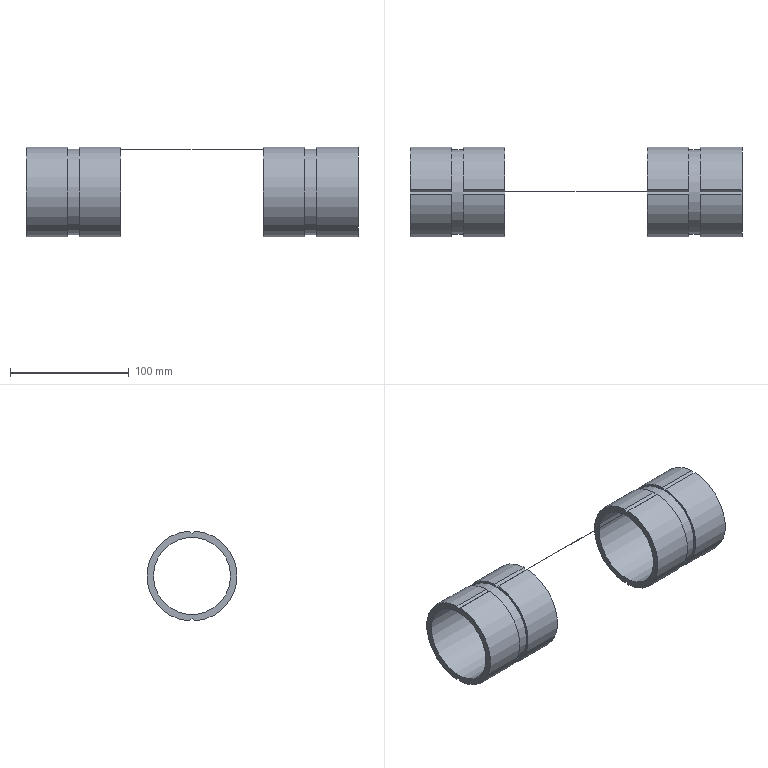Part | NX | features MAIN_BODY 2 | 1 solid | 44 faces | box 280 x 76 x 75.9 mm | volume 184505 mm3 | plane 32 | cylinder 12 | commonest cylinder face diameters 76 x8 65 x2 72 x2
STEP:
#1=CARTESIAN_POINT('',(1430.,847.5,-280.));
#2=VERTEX_POINT('',#1);
#3=CARTESIAN_POINT('',(1430.,880.,-280.));
#4=DIRECTION('',(-1.,0.,0.));
#5=DIRECTION('',(0.,-1.,0.));
#6=AXIS2_PLACEMENT_3D('',#3,#4,#5);
#7=CIRCLE('',#6,32.5);
#8=EDGE_CURVE('',#2,#2,#7,.F.);
#9=ORIENTED_EDGE('',*,*,#8,.T.);
#10=EDGE_LOOP('',(#9));
#11=FACE_BOUND('',#10,.T.);
#12=CARTESIAN_POINT('',(1430.,880.05,-244.));
#13=VERTEX_POINT('',#12);
#14=CARTESIAN_POINT('',(1430.,880.05,-244.05));
#15=VERTEX_POINT('',#14);
#16=CARTESIAN_POINT('',(1430.,880.05,-280.));
#17=DIRECTION('',(0.,0.,1.));
#18=VECTOR('',#17,1000.);
#19=LINE('',#16,#18);
#20=EDGE_CURVE('',#13,#15,#19,.F.);
#21=ORIENTED_EDGE('',*,*,#20,.F.);
#22=CARTESIAN_POINT('',(1430.,880.,-244.));
#23=VERTEX_POINT('',#22);
#24=CARTESIAN_POINT('',(1430.,880.,-244.));
#25=DIRECTION('',(0.,1.,0.));
#26=VECTOR('',#25,1000.);
#27=LINE('',#24,#26);
#28=EDGE_CURVE('',#13,#23,#27,.F.);
#29=ORIENTED_EDGE('',*,*,#28,.T.);
#30=CARTESIAN_POINT('',(1430.,881.95,-242.05));
#31=VERTEX_POINT('',#30);
#32=CARTESIAN_POINT('',(1430.,862.,-262.));
#33=DIRECTION('',(0.,-0.7071,-0.7071));
#34=VECTOR('',#33,1000.);
#35=LINE('',#32,#34);
#36=EDGE_CURVE('',#23,#31,#35,.F.);
#37=ORIENTED_EDGE('',*,*,#36,.T.);
#38=CARTESIAN_POINT('',(1430.,881.95,-317.95));
#39=VERTEX_POINT('',#38);
#40=CARTESIAN_POINT('',(1430.,880.,-280.));
#41=DIRECTION('',(1.,0.,0.));
#42=DIRECTION('',(0.,1.,0.));
#43=AXIS2_PLACEMENT_3D('',#40,#41,#42);
#44=CIRCLE('',#43,38.);
#45=EDGE_CURVE('',#39,#31,#44,.T.);
#46=ORIENTED_EDGE('',*,*,#45,.F.);
#47=CARTESIAN_POINT('',(1430.,880.,-316.));
#48=VERTEX_POINT('',#47);
#49=CARTESIAN_POINT('',(1430.,862.,-298.));
#50=DIRECTION('',(0.,-0.7071,0.7071));
#51=VECTOR('',#50,1000.);
#52=LINE('',#49,#51);
#53=EDGE_CURVE('',#48,#39,#52,.F.);
#54=ORIENTED_EDGE('',*,*,#53,.F.);
#55=CARTESIAN_POINT('',(1430.,878.05,-317.95));
#56=VERTEX_POINT('',#55);
#57=CARTESIAN_POINT('',(1430.,898.,-298.));
#58=DIRECTION('',(0.,-0.7071,-0.7071));
#59=VECTOR('',#58,1000.);
#60=LINE('',#57,#59);
#61=EDGE_CURVE('',#56,#48,#60,.F.);
#62=ORIENTED_EDGE('',*,*,#61,.F.);
#63=CARTESIAN_POINT('',(1430.,878.05,-242.05));
#64=VERTEX_POINT('',#63);
#65=CARTESIAN_POINT('',(1430.,880.,-280.));
#66=DIRECTION('',(1.,0.,0.));
#67=DIRECTION('',(0.,1.,0.));
#68=AXIS2_PLACEMENT_3D('',#65,#66,#67);
#69=CIRCLE('',#68,38.);
#70=EDGE_CURVE('',#64,#56,#69,.T.);
#71=ORIENTED_EDGE('',*,*,#70,.F.);
#72=CARTESIAN_POINT('',(1430.,898.,-262.));
#73=DIRECTION('',(0.,-0.7071,0.7071));
#74=VECTOR('',#73,1000.);
#75=LINE('',#72,#74);
#76=EDGE_CURVE('',#64,#23,#75,.F.);
#77=ORIENTED_EDGE('',*,*,#76,.T.);
#78=CARTESIAN_POINT('',(1430.,879.95,-244.));
#79=VERTEX_POINT('',#78);
#80=CARTESIAN_POINT('',(1430.,880.,-244.));
#81=DIRECTION('',(0.,1.,0.));
#82=VECTOR('',#81,1000.);
#83=LINE('',#80,#82);
#84=EDGE_CURVE('',#23,#79,#83,.F.);
#85=ORIENTED_EDGE('',*,*,#84,.T.);
#86=CARTESIAN_POINT('',(1430.,879.95,-244.05));
#87=VERTEX_POINT('',#86);
#88=CARTESIAN_POINT('',(1430.,879.95,-280.));
#89=DIRECTION('',(0.,0.,1.));
#90=VECTOR('',#89,1000.);
#91=LINE('',#88,#90);
#92=EDGE_CURVE('',#79,#87,#91,.F.);
#93=ORIENTED_EDGE('',*,*,#92,.T.);
#94=CARTESIAN_POINT('',(1430.,880.,-244.05));
#95=DIRECTION('',(0.,1.,0.));
#96=VECTOR('',#95,1000.);
#97=LINE('',#94,#96);
#98=EDGE_CURVE('',#87,#15,#97,.T.);
#99=ORIENTED_EDGE('',*,*,#98,.T.);
#100=EDGE_LOOP('',(#21,#29,#37,#46,#54,#62,#71,#77,#85,#93,#99));
#101=FACE_BOUND('',#100,.T.);
#102=CARTESIAN_POINT('',(1430.,880.,-280.));
#103=DIRECTION('',(-1.,0.,0.));
#104=DIRECTION('',(0.,-1.,0.));
#105=AXIS2_PLACEMENT_3D('',#102,#103,#104);
#106=PLANE('',#105);
#107=ADVANCED_FACE('',(#11,#101),#106,.T.);
#108=CARTESIAN_POINT('',(1475.,881.95,-317.95));
#109=VERTEX_POINT('',#108);
#110=CARTESIAN_POINT('',(1510.,881.95,-317.95));
#111=VERTEX_POINT('',#110);
#112=CARTESIAN_POINT('',(1510.,881.95,-317.95));
#113=DIRECTION('',(-1.,0.,0.));
#114=VECTOR('',#113,1000.);
#115=LINE('',#112,#114);
#116=EDGE_CURVE('',#109,#111,#115,.F.);
#117=ORIENTED_EDGE('',*,*,#116,.F.);
#118=CARTESIAN_POINT('',(1475.,881.95,-242.05));
#119=VERTEX_POINT('',#118);
#120=CARTESIAN_POINT('',(1475.,880.,-280.));
#121=DIRECTION('',(-1.,0.,0.));
#122=DIRECTION('',(0.,-1.,0.));
#123=AXIS2_PLACEMENT_3D('',#120,#121,#122);
#124=CIRCLE('',#123,38.);
#125=EDGE_CURVE('',#119,#109,#124,.T.);
#126=ORIENTED_EDGE('',*,*,#125,.F.);
#127=CARTESIAN_POINT('',(1510.,881.95,-242.05));
#128=VERTEX_POINT('',#127);
#129=CARTESIAN_POINT('',(1510.,881.95,-242.05));
#130=DIRECTION('',(-1.,0.,0.));
#131=VECTOR('',#130,1000.);
#132=LINE('',#129,#131);
#133=EDGE_CURVE('',#119,#128,#132,.F.);
#134=ORIENTED_EDGE('',*,*,#133,.T.);
#135=CARTESIAN_POINT('',(1510.,880.,-280.));
#136=DIRECTION('',(1.,0.,0.));
#137=DIRECTION('',(0.,1.,0.));
#138=AXIS2_PLACEMENT_3D('',#135,#136,#137);
#139=CIRCLE('',#138,38.);
#140=EDGE_CURVE('',#111,#128,#139,.T.);
#141=ORIENTED_EDGE('',*,*,#140,.F.);
#142=EDGE_LOOP('',(#117,#126,#134,#141));
#143=FACE_BOUND('',#142,.T.);
#144=CARTESIAN_POINT('',(1510.,880.,-280.));
#145=DIRECTION('',(-1.,0.,0.));
#146=DIRECTION('',(0.,-1.,0.));
#147=AXIS2_PLACEMENT_3D('',#144,#145,#146);
#148=CYLINDRICAL_SURFACE('',#147,38.);
#149=ADVANCED_FACE('',(#143),#148,.T.);
#150=CARTESIAN_POINT('',(1510.,878.05,-317.95));
#151=VERTEX_POINT('',#150);
#152=CARTESIAN_POINT('',(1475.,878.05,-317.95));
#153=VERTEX_POINT('',#152);
#154=CARTESIAN_POINT('',(1510.,878.05,-317.95));
#155=DIRECTION('',(-1.,0.,0.));
#156=VECTOR('',#155,1000.);
#157=LINE('',#154,#156);
#158=EDGE_CURVE('',#151,#153,#157,.T.);
#159=ORIENTED_EDGE('',*,*,#158,.F.);
#160=CARTESIAN_POINT('',(1510.,878.05,-242.05));
#161=VERTEX_POINT('',#160);
#162=CARTESIAN_POINT('',(1510.,880.,-280.));
#163=DIRECTION('',(1.,0.,0.));
#164=DIRECTION('',(0.,1.,0.));
#165=AXIS2_PLACEMENT_3D('',#162,#163,#164);
#166=CIRCLE('',#165,38.);
#167=EDGE_CURVE('',#161,#151,#166,.T.);
#168=ORIENTED_EDGE('',*,*,#167,.F.);
#169=CARTESIAN_POINT('',(1475.,878.05,-242.05));
#170=VERTEX_POINT('',#169);
#171=CARTESIAN_POINT('',(1510.,878.05,-242.05));
#172=DIRECTION('',(-1.,0.,0.));
#173=VECTOR('',#172,1000.);
#174=LINE('',#171,#173);
#175=EDGE_CURVE('',#161,#170,#174,.T.);
#176=ORIENTED_EDGE('',*,*,#175,.T.);
#177=CARTESIAN_POINT('',(1475.,880.,-280.));
#178=DIRECTION('',(-1.,0.,0.));
#179=DIRECTION('',(0.,-1.,0.));
#180=AXIS2_PLACEMENT_3D('',#177,#178,#179);
#181=CIRCLE('',#180,38.);
#182=EDGE_CURVE('',#153,#170,#181,.T.);
#183=ORIENTED_EDGE('',*,*,#182,.F.);
#184=EDGE_LOOP('',(#159,#168,#176,#183));
#185=FACE_BOUND('',#184,.T.);
#186=CARTESIAN_POINT('',(1510.,880.,-280.));
#187=DIRECTION('',(-1.,0.,0.));
#188=DIRECTION('',(0.,-1.,0.));
#189=AXIS2_PLACEMENT_3D('',#186,#187,#188);
#190=CYLINDRICAL_SURFACE('',#189,38.);
#191=ADVANCED_FACE('',(#185),#190,.T.);
#192=CARTESIAN_POINT('',(1510.,847.5,-280.));
#193=VERTEX_POINT('',#192);
#194=CARTESIAN_POINT('',(1510.,880.,-280.));
#195=DIRECTION('',(-1.,0.,0.));
#196=DIRECTION('',(0.,-1.,0.));
#197=AXIS2_PLACEMENT_3D('',#194,#195,#196);
#198=CIRCLE('',#197,32.5);
#199=EDGE_CURVE('',#193,#193,#198,.F.);
#200=ORIENTED_EDGE('',*,*,#199,.F.);
#201=EDGE_LOOP('',(#200));
#202=FACE_BOUND('',#201,.T.);
#203=CARTESIAN_POINT('',(1510.,880.,-316.));
#204=VERTEX_POINT('',#203);
#205=CARTESIAN_POINT('',(1510.,862.,-298.));
#206=DIRECTION('',(0.,-0.7071,0.7071));
#207=VECTOR('',#206,1000.);
#208=LINE('',#205,#207);
#209=EDGE_CURVE('',#111,#204,#208,.T.);
#210=ORIENTED_EDGE('',*,*,#209,.F.);
#211=ORIENTED_EDGE('',*,*,#140,.T.);
#212=CARTESIAN_POINT('',(1510.,880.,-244.));
#213=VERTEX_POINT('',#212);
#214=CARTESIAN_POINT('',(1510.,862.,-262.));
#215=DIRECTION('',(0.,-0.7071,-0.7071));
#216=VECTOR('',#215,1000.);
#217=LINE('',#214,#216);
#218=EDGE_CURVE('',#128,#213,#217,.T.);
#219=ORIENTED_EDGE('',*,*,#218,.T.);
#220=CARTESIAN_POINT('',(1510.,898.,-262.));
#221=DIRECTION('',(0.,-0.7071,0.7071));
#222=VECTOR('',#221,1000.);
#223=LINE('',#220,#222);
#224=EDGE_CURVE('',#213,#161,#223,.T.);
#225=ORIENTED_EDGE('',*,*,#224,.T.);
#226=ORIENTED_EDGE('',*,*,#167,.T.);
#227=CARTESIAN_POINT('',(1510.,898.,-298.));
#228=DIRECTION('',(0.,-0.7071,-0.7071));
#229=VECTOR('',#228,1000.);
#230=LINE('',#227,#229);
#231=EDGE_CURVE('',#204,#151,#230,.T.);
#232=ORIENTED_EDGE('',*,*,#231,.F.);
#233=EDGE_LOOP('',(#210,#211,#219,#225,#226,#232));
#234=FACE_BOUND('',#233,.T.);
#235=CARTESIAN_POINT('',(1510.,880.,-280.));
#236=DIRECTION('',(-1.,0.,0.));
#237=DIRECTION('',(0.,-1.,0.));
#238=AXIS2_PLACEMENT_3D('',#235,#236,#237);
#239=PLANE('',#238);
#240=ADVANCED_FACE('',(#202,#234),#239,.F.);
#241=CARTESIAN_POINT('',(1465.,881.95,-317.95));
#242=VERTEX_POINT('',#241);
#243=CARTESIAN_POINT('',(1510.,881.95,-317.95));
#244=DIRECTION('',(-1.,0.,0.));
#245=VECTOR('',#244,1000.);
#246=LINE('',#243,#245);
#247=EDGE_CURVE('',#39,#242,#246,.F.);
#248=ORIENTED_EDGE('',*,*,#247,.F.);
#249=ORIENTED_EDGE('',*,*,#45,.T.);
#250=CARTESIAN_POINT('',(1465.,881.95,-242.05));
#251=VERTEX_POINT('',#250);
#252=CARTESIAN_POINT('',(1510.,881.95,-242.05));
#253=DIRECTION('',(-1.,0.,0.));
#254=VECTOR('',#253,1000.);
#255=LINE('',#252,#254);
#256=EDGE_CURVE('',#31,#251,#255,.F.);
#257=ORIENTED_EDGE('',*,*,#256,.T.);
#258=CARTESIAN_POINT('',(1465.,880.,-280.));
#259=DIRECTION('',(-1.,0.,0.));
#260=DIRECTION('',(0.,-1.,0.));
#261=AXIS2_PLACEMENT_3D('',#258,#259,#260);
#262=CIRCLE('',#261,38.);
#263=EDGE_CURVE('',#251,#242,#262,.T.);
#264=ORIENTED_EDGE('',*,*,#263,.T.);
#265=EDGE_LOOP('',(#248,#249,#257,#264));
#266=FACE_BOUND('',#265,.T.);
#267=CARTESIAN_POINT('',(1510.,880.,-280.));
#268=DIRECTION('',(-1.,0.,0.));
#269=DIRECTION('',(0.,-1.,0.));
#270=AXIS2_PLACEMENT_3D('',#267,#268,#269);
#271=CYLINDRICAL_SURFACE('',#270,38.);
#272=ADVANCED_FACE('',(#266),#271,.T.);
#273=CARTESIAN_POINT('',(1465.,878.05,-317.95));
#274=VERTEX_POINT('',#273);
#275=CARTESIAN_POINT('',(1510.,878.05,-317.95));
#276=DIRECTION('',(-1.,0.,0.));
#277=VECTOR('',#276,1000.);
#278=LINE('',#275,#277);
#279=EDGE_CURVE('',#274,#56,#278,.T.);
#280=ORIENTED_EDGE('',*,*,#279,.F.);
#281=CARTESIAN_POINT('',(1465.,878.05,-242.05));
#282=VERTEX_POINT('',#281);
#283=CARTESIAN_POINT('',(1465.,880.,-280.));
#284=DIRECTION('',(-1.,0.,0.));
#285=DIRECTION('',(0.,-1.,0.));
#286=AXIS2_PLACEMENT_3D('',#283,#284,#285);
#287=CIRCLE('',#286,38.);
#288=EDGE_CURVE('',#274,#282,#287,.T.);
#289=ORIENTED_EDGE('',*,*,#288,.T.);
#290=CARTESIAN_POINT('',(1510.,878.05,-242.05));
#291=DIRECTION('',(-1.,0.,0.));
#292=VECTOR('',#291,1000.);
#293=LINE('',#290,#292);
#294=EDGE_CURVE('',#282,#64,#293,.T.);
#295=ORIENTED_EDGE('',*,*,#294,.T.);
#296=ORIENTED_EDGE('',*,*,#70,.T.);
#297=EDGE_LOOP('',(#280,#289,#295,#296));
#298=FACE_BOUND('',#297,.T.);
#299=CARTESIAN_POINT('',(1510.,880.,-280.));
#300=DIRECTION('',(-1.,0.,0.));
#301=DIRECTION('',(0.,-1.,0.));
#302=AXIS2_PLACEMENT_3D('',#299,#300,#301);
#303=CYLINDRICAL_SURFACE('',#302,38.);
#304=ADVANCED_FACE('',(#298),#303,.T.);
#305=CARTESIAN_POINT('',(1475.,880.,-316.));
#306=VERTEX_POINT('',#305);
#307=CARTESIAN_POINT('',(1475.,843.,-279.));
#308=DIRECTION('',(0.,0.7071,-0.7071));
#309=VECTOR('',#308,1000.);
#310=LINE('',#307,#309);
#311=EDGE_CURVE('',#306,#109,#310,.T.);
#312=ORIENTED_EDGE('',*,*,#311,.F.);
#313=CARTESIAN_POINT('',(1475.,880.,-244.));
#314=VERTEX_POINT('',#313);
#315=CARTESIAN_POINT('',(1475.,880.,-280.));
#316=DIRECTION('',(-1.,0.,0.));
#317=DIRECTION('',(0.,-1.,0.));
#318=AXIS2_PLACEMENT_3D('',#315,#316,#317);
#319=CIRCLE('',#318,36.);
#320=EDGE_CURVE('',#314,#306,#319,.T.);
#321=ORIENTED_EDGE('',*,*,#320,.F.);
#322=CARTESIAN_POINT('',(1475.,881.,-243.));
#323=DIRECTION('',(0.,0.7071,0.7071));
#324=VECTOR('',#323,1000.);
#325=LINE('',#322,#324);
#326=EDGE_CURVE('',#314,#119,#325,.T.);
#327=ORIENTED_EDGE('',*,*,#326,.T.);
#328=ORIENTED_EDGE('',*,*,#125,.T.);
#329=EDGE_LOOP('',(#312,#321,#327,#328));
#330=FACE_BOUND('',#329,.T.);
#331=CARTESIAN_POINT('',(1475.,880.,-242.));
#332=DIRECTION('',(1.,0.,0.));
#333=DIRECTION('',(0.,1.,0.));
#334=AXIS2_PLACEMENT_3D('',#331,#332,#333);
#335=PLANE('',#334);
#336=ADVANCED_FACE('',(#330),#335,.F.);
#337=CARTESIAN_POINT('',(1475.,917.,-279.));
#338=DIRECTION('',(0.,0.7071,0.7071));
#339=VECTOR('',#338,1000.);
#340=LINE('',#337,#339);
#341=EDGE_CURVE('',#153,#306,#340,.T.);
#342=ORIENTED_EDGE('',*,*,#341,.F.);
#343=ORIENTED_EDGE('',*,*,#182,.T.);
#344=CARTESIAN_POINT('',(1475.,879.,-243.));
#345=DIRECTION('',(0.,0.7071,-0.7071));
#346=VECTOR('',#345,1000.);
#347=LINE('',#344,#346);
#348=EDGE_CURVE('',#170,#314,#347,.T.);
#349=ORIENTED_EDGE('',*,*,#348,.T.);
#350=CARTESIAN_POINT('',(1475.,880.,-280.));
#351=DIRECTION('',(-1.,0.,0.));
#352=DIRECTION('',(0.,-1.,0.));
#353=AXIS2_PLACEMENT_3D('',#350,#351,#352);
#354=CIRCLE('',#353,36.);
#355=EDGE_CURVE('',#306,#314,#354,.T.);
#356=ORIENTED_EDGE('',*,*,#355,.F.);
#357=EDGE_LOOP('',(#342,#343,#349,#356));
#358=FACE_BOUND('',#357,.T.);
#359=CARTESIAN_POINT('',(1475.,880.,-242.));
#360=DIRECTION('',(1.,0.,0.));
#361=DIRECTION('',(0.,1.,0.));
#362=AXIS2_PLACEMENT_3D('',#359,#360,#361);
#363=PLANE('',#362);
#364=ADVANCED_FACE('',(#358),#363,.F.);
#365=CARTESIAN_POINT('',(1465.,880.,-244.));
#366=VERTEX_POINT('',#365);
#367=CARTESIAN_POINT('',(1465.,880.,-244.));
#368=DIRECTION('',(0.,-0.7071,-0.7071));
#369=VECTOR('',#368,1000.);
#370=LINE('',#367,#369);
#371=EDGE_CURVE('',#251,#366,#370,.T.);
#372=ORIENTED_EDGE('',*,*,#371,.T.);
#373=CARTESIAN_POINT('',(1465.,880.,-316.));
#374=VERTEX_POINT('',#373);
#375=CARTESIAN_POINT('',(1465.,880.,-280.));
#376=DIRECTION('',(-1.,0.,0.));
#377=DIRECTION('',(0.,-1.,0.));
#378=AXIS2_PLACEMENT_3D('',#375,#376,#377);
#379=CIRCLE('',#378,36.);
#380=EDGE_CURVE('',#366,#374,#379,.T.);
#381=ORIENTED_EDGE('',*,*,#380,.T.);
#382=CARTESIAN_POINT('',(1465.,844.,-280.));
#383=DIRECTION('',(0.,-0.7071,0.7071));
#384=VECTOR('',#383,1000.);
#385=LINE('',#382,#384);
#386=EDGE_CURVE('',#242,#374,#385,.T.);
#387=ORIENTED_EDGE('',*,*,#386,.F.);
#388=ORIENTED_EDGE('',*,*,#263,.F.);
#389=EDGE_LOOP('',(#372,#381,#387,#388));
#390=FACE_BOUND('',#389,.T.);
#391=CARTESIAN_POINT('',(1465.,880.,-244.));
#392=DIRECTION('',(-1.,0.,0.));
#393=DIRECTION('',(0.,-1.,0.));
#394=AXIS2_PLACEMENT_3D('',#391,#392,#393);
#395=PLANE('',#394);
#396=ADVANCED_FACE('',(#390),#395,.F.);
#397=CARTESIAN_POINT('',(1465.,880.,-280.));
#398=DIRECTION('',(-1.,0.,0.));
#399=DIRECTION('',(0.,-1.,0.));
#400=AXIS2_PLACEMENT_3D('',#397,#398,#399);
#401=CIRCLE('',#400,36.);
#402=EDGE_CURVE('',#374,#366,#401,.T.);
#403=ORIENTED_EDGE('',*,*,#402,.T.);
#404=CARTESIAN_POINT('',(1465.,880.,-244.));
#405=DIRECTION('',(0.,-0.7071,0.7071));
#406=VECTOR('',#405,1000.);
#407=LINE('',#404,#406);
#408=EDGE_CURVE('',#366,#282,#407,.T.);
#409=ORIENTED_EDGE('',*,*,#408,.T.);
#410=ORIENTED_EDGE('',*,*,#288,.F.);
#411=CARTESIAN_POINT('',(1465.,916.,-280.));
#412=DIRECTION('',(0.,-0.7071,-0.7071));
#413=VECTOR('',#412,1000.);
#414=LINE('',#411,#413);
#415=EDGE_CURVE('',#374,#274,#414,.T.);
#416=ORIENTED_EDGE('',*,*,#415,.F.);
#417=EDGE_LOOP('',(#403,#409,#410,#416));
#418=FACE_BOUND('',#417,.T.);
#419=CARTESIAN_POINT('',(1465.,880.,-244.));
#420=DIRECTION('',(-1.,0.,0.));
#421=DIRECTION('',(0.,-1.,0.));
#422=AXIS2_PLACEMENT_3D('',#419,#420,#421);
#423=PLANE('',#422);
#424=ADVANCED_FACE('',(#418),#423,.F.);
#425=ORIENTED_EDGE('',*,*,#8,.F.);
#426=EDGE_LOOP('',(#425));
#427=FACE_BOUND('',#426,.T.);
#428=ORIENTED_EDGE('',*,*,#199,.T.);
#429=EDGE_LOOP('',(#428));
#430=FACE_BOUND('',#429,.T.);
#431=CARTESIAN_POINT('',(1510.,880.,-280.));
#432=DIRECTION('',(-1.,0.,0.));
#433=DIRECTION('',(0.,-1.,0.));
#434=AXIS2_PLACEMENT_3D('',#431,#432,#433);
#435=CYLINDRICAL_SURFACE('',#434,32.5);
#436=ADVANCED_FACE('',(#427,#430),#435,.F.);
#437=ORIENTED_EDGE('',*,*,#402,.F.);
#438=ORIENTED_EDGE('',*,*,#380,.F.);
#439=EDGE_LOOP('',(#437,#438));
#440=FACE_BOUND('',#439,.T.);
#441=ORIENTED_EDGE('',*,*,#320,.T.);
#442=ORIENTED_EDGE('',*,*,#355,.T.);
#443=EDGE_LOOP('',(#441,#442));
#444=FACE_BOUND('',#443,.T.);
#445=CARTESIAN_POINT('',(1530.2,880.,-280.));
#446=DIRECTION('',(-1.,0.,0.));
#447=DIRECTION('',(0.,-1.,0.));
#448=AXIS2_PLACEMENT_3D('',#445,#446,#447);
#449=CYLINDRICAL_SURFACE('',#448,36.);
#450=ADVANCED_FACE('',(#440,#444),#449,.T.);
#451=CARTESIAN_POINT('',(1090.,880.,-244.));
#452=DIRECTION('',(1.,0.,0.));
#453=VECTOR('',#452,1000.);
#454=LINE('',#451,#453);
#455=EDGE_CURVE('',#23,#366,#454,.T.);
#456=ORIENTED_EDGE('',*,*,#455,.T.);
#457=ORIENTED_EDGE('',*,*,#371,.F.);
#458=ORIENTED_EDGE('',*,*,#256,.F.);
#459=ORIENTED_EDGE('',*,*,#36,.F.);
#460=EDGE_LOOP('',(#456,#457,#458,#459));
#461=FACE_BOUND('',#460,.T.);
#462=CARTESIAN_POINT('',(1090.,880.,-244.));
#463=DIRECTION('',(0.,0.7071,-0.7071));
#464=DIRECTION('',(0.,0.7071,0.7071));
#465=AXIS2_PLACEMENT_3D('',#462,#463,#464);
#466=PLANE('',#465);
#467=ADVANCED_FACE('',(#461),#466,.F.);
#468=ORIENTED_EDGE('',*,*,#294,.F.);
#469=ORIENTED_EDGE('',*,*,#408,.F.);
#470=ORIENTED_EDGE('',*,*,#455,.F.);
#471=ORIENTED_EDGE('',*,*,#76,.F.);
#472=EDGE_LOOP('',(#468,#469,#470,#471));
#473=FACE_BOUND('',#472,.T.);
#474=CARTESIAN_POINT('',(1090.,870.,-234.));
#475=DIRECTION('',(0.,-0.7071,-0.7071));
#476=DIRECTION('',(0.,0.7071,-0.7071));
#477=AXIS2_PLACEMENT_3D('',#474,#475,#476);
#478=PLANE('',#477);
#479=ADVANCED_FACE('',(#473),#478,.F.);
#480=CARTESIAN_POINT('',(1090.,880.,-244.));
#481=DIRECTION('',(1.,0.,0.));
#482=VECTOR('',#481,1000.);
#483=LINE('',#480,#482);
#484=EDGE_CURVE('',#314,#213,#483,.T.);
#485=ORIENTED_EDGE('',*,*,#484,.F.);
#486=ORIENTED_EDGE('',*,*,#348,.F.);
#487=ORIENTED_EDGE('',*,*,#175,.F.);
#488=ORIENTED_EDGE('',*,*,#224,.F.);
#489=EDGE_LOOP('',(#485,#486,#487,#488));
#490=FACE_BOUND('',#489,.T.);
#491=CARTESIAN_POINT('',(1090.,870.,-234.));
#492=DIRECTION('',(0.,-0.7071,-0.7071));
#493=DIRECTION('',(0.,0.7071,-0.7071));
#494=AXIS2_PLACEMENT_3D('',#491,#492,#493);
#495=PLANE('',#494);
#496=ADVANCED_FACE('',(#490),#495,.F.);
#497=ORIENTED_EDGE('',*,*,#133,.F.);
#498=ORIENTED_EDGE('',*,*,#326,.F.);
#499=ORIENTED_EDGE('',*,*,#484,.T.);
#500=ORIENTED_EDGE('',*,*,#218,.F.);
#501=EDGE_LOOP('',(#497,#498,#499,#500));
#502=FACE_BOUND('',#501,.T.);
#503=CARTESIAN_POINT('',(1090.,880.,-244.));
#504=DIRECTION('',(0.,0.7071,-0.7071));
#505=DIRECTION('',(0.,0.7071,0.7071));
#506=AXIS2_PLACEMENT_3D('',#503,#504,#505);
#507=PLANE('',#506);
#508=ADVANCED_FACE('',(#502),#507,.F.);
#509=ORIENTED_EDGE('',*,*,#61,.T.);
#510=CARTESIAN_POINT('',(590.,880.,-316.));
#511=DIRECTION('',(1.,0.,0.));
#512=VECTOR('',#511,1000.);
#513=LINE('',#510,#512);
#514=EDGE_CURVE('',#48,#374,#513,.T.);
#515=ORIENTED_EDGE('',*,*,#514,.T.);
#516=ORIENTED_EDGE('',*,*,#415,.T.);
#517=ORIENTED_EDGE('',*,*,#279,.T.);
#518=EDGE_LOOP('',(#509,#515,#516,#517));
#519=FACE_BOUND('',#518,.T.);
#520=CARTESIAN_POINT('',(590.,870.,-326.));
#521=DIRECTION('',(0.,0.7071,-0.7071));
#522=DIRECTION('',(0.,0.7071,0.7071));
#523=AXIS2_PLACEMENT_3D('',#520,#521,#522);
#524=PLANE('',#523);
#525=ADVANCED_FACE('',(#519),#524,.T.);
#526=ORIENTED_EDGE('',*,*,#53,.T.);
#527=ORIENTED_EDGE('',*,*,#247,.T.);
#528=ORIENTED_EDGE('',*,*,#386,.T.);
#529=ORIENTED_EDGE('',*,*,#514,.F.);
#530=EDGE_LOOP('',(#526,#527,#528,#529));
#531=FACE_BOUND('',#530,.T.);
#532=CARTESIAN_POINT('',(590.,880.,-316.));
#533=DIRECTION('',(0.,-0.7071,-0.7071));
#534=DIRECTION('',(0.,0.7071,-0.7071));
#535=AXIS2_PLACEMENT_3D('',#532,#533,#534);
#536=PLANE('',#535);
#537=ADVANCED_FACE('',(#531),#536,.T.);
#538=ORIENTED_EDGE('',*,*,#209,.T.);
#539=CARTESIAN_POINT('',(590.,880.,-316.));
#540=DIRECTION('',(1.,0.,0.));
#541=VECTOR('',#540,1000.);
#542=LINE('',#539,#541);
#543=EDGE_CURVE('',#306,#204,#542,.T.);
#544=ORIENTED_EDGE('',*,*,#543,.F.);
#545=ORIENTED_EDGE('',*,*,#311,.T.);
#546=ORIENTED_EDGE('',*,*,#116,.T.);
#547=EDGE_LOOP('',(#538,#544,#545,#546));
#548=FACE_BOUND('',#547,.T.);
#549=CARTESIAN_POINT('',(590.,880.,-316.));
#550=DIRECTION('',(0.,-0.7071,-0.7071));
#551=DIRECTION('',(0.,0.7071,-0.7071));
#552=AXIS2_PLACEMENT_3D('',#549,#550,#551);
#553=PLANE('',#552);
#554=ADVANCED_FACE('',(#548),#553,.T.);
#555=ORIENTED_EDGE('',*,*,#231,.T.);
#556=ORIENTED_EDGE('',*,*,#158,.T.);
#557=ORIENTED_EDGE('',*,*,#341,.T.);
#558=ORIENTED_EDGE('',*,*,#543,.T.);
#559=EDGE_LOOP('',(#555,#556,#557,#558));
#560=FACE_BOUND('',#559,.T.);
#561=CARTESIAN_POINT('',(590.,870.,-326.));
#562=DIRECTION('',(0.,0.7071,-0.7071));
#563=DIRECTION('',(0.,0.7071,0.7071));
#564=AXIS2_PLACEMENT_3D('',#561,#562,#563);
#565=PLANE('',#564);
#566=ADVANCED_FACE('',(#560),#565,.T.);
#567=ORIENTED_EDGE('',*,*,#98,.F.);
#568=CARTESIAN_POINT('',(1310.,879.95,-244.05));
#569=VERTEX_POINT('',#568);
#570=CARTESIAN_POINT('',(1465.,879.95,-244.05));
#571=DIRECTION('',(1.,0.,0.));
#572=VECTOR('',#571,1000.);
#573=LINE('',#570,#572);
#574=EDGE_CURVE('',#87,#569,#573,.F.);
#575=ORIENTED_EDGE('',*,*,#574,.T.);
#576=CARTESIAN_POINT('',(1310.,880.05,-244.05));
#577=VERTEX_POINT('',#576);
#578=CARTESIAN_POINT('',(1310.,880.,-244.05));
#579=DIRECTION('',(0.,-1.,0.));
#580=VECTOR('',#579,1000.);
#581=LINE('',#578,#580);
#582=EDGE_CURVE('',#569,#577,#581,.F.);
#583=ORIENTED_EDGE('',*,*,#582,.T.);
#584=CARTESIAN_POINT('',(1465.,880.05,-244.05));
#585=DIRECTION('',(1.,0.,0.));
#586=VECTOR('',#585,1000.);
#587=LINE('',#584,#586);
#588=EDGE_CURVE('',#15,#577,#587,.F.);
#589=ORIENTED_EDGE('',*,*,#588,.F.);
#590=EDGE_LOOP('',(#567,#575,#583,#589));
#591=FACE_BOUND('',#590,.T.);
#592=CARTESIAN_POINT('',(1465.,880.,-244.05));
#593=DIRECTION('',(0.,0.,1.));
#594=DIRECTION('',(-1.,0.,0.));
#595=AXIS2_PLACEMENT_3D('',#592,#593,#594);
#596=PLANE('',#595);
#597=ADVANCED_FACE('',(#591),#596,.F.);
#598=CARTESIAN_POINT('',(1310.,880.05,-244.));
#599=VERTEX_POINT('',#598);
#600=CARTESIAN_POINT('',(1465.,880.05,-244.));
#601=DIRECTION('',(1.,0.,0.));
#602=VECTOR('',#601,1000.);
#603=LINE('',#600,#602);
#604=EDGE_CURVE('',#13,#599,#603,.F.);
#605=ORIENTED_EDGE('',*,*,#604,.F.);
#606=ORIENTED_EDGE('',*,*,#20,.T.);
#607=ORIENTED_EDGE('',*,*,#588,.T.);
#608=CARTESIAN_POINT('',(1310.,880.05,-244.));
#609=DIRECTION('',(0.,0.,-1.));
#610=VECTOR('',#609,1000.);
#611=LINE('',#608,#610);
#612=EDGE_CURVE('',#599,#577,#611,.T.);
#613=ORIENTED_EDGE('',*,*,#612,.F.);
#614=EDGE_LOOP('',(#605,#606,#607,#613));
#615=FACE_BOUND('',#614,.T.);
#616=CARTESIAN_POINT('',(1465.,880.05,-244.));
#617=DIRECTION('',(0.,-1.,0.));
#618=DIRECTION('',(1.,0.,0.));
#619=AXIS2_PLACEMENT_3D('',#616,#617,#618);
#620=PLANE('',#619);
#621=ADVANCED_FACE('',(#615),#620,.F.);
#622=ORIENTED_EDGE('',*,*,#92,.F.);
#623=CARTESIAN_POINT('',(1310.,879.95,-244.));
#624=VERTEX_POINT('',#623);
#625=CARTESIAN_POINT('',(1465.,879.95,-244.));
#626=DIRECTION('',(1.,0.,0.));
#627=VECTOR('',#626,1000.);
#628=LINE('',#625,#627);
#629=EDGE_CURVE('',#79,#624,#628,.F.);
#630=ORIENTED_EDGE('',*,*,#629,.T.);
#631=CARTESIAN_POINT('',(1310.,879.95,-244.));
#632=DIRECTION('',(0.,0.,-1.));
#633=VECTOR('',#632,1000.);
#634=LINE('',#631,#633);
#635=EDGE_CURVE('',#624,#569,#634,.T.);
#636=ORIENTED_EDGE('',*,*,#635,.T.);
#637=ORIENTED_EDGE('',*,*,#574,.F.);
#638=EDGE_LOOP('',(#622,#630,#636,#637));
#639=FACE_BOUND('',#638,.T.);
#640=CARTESIAN_POINT('',(1465.,879.95,-244.));
#641=DIRECTION('',(0.,-1.,0.));
#642=DIRECTION('',(1.,0.,0.));
#643=AXIS2_PLACEMENT_3D('',#640,#641,#642);
#644=PLANE('',#643);
#645=ADVANCED_FACE('',(#639),#644,.T.);
#646=ORIENTED_EDGE('',*,*,#28,.F.);
#647=ORIENTED_EDGE('',*,*,#604,.T.);
#648=CARTESIAN_POINT('',(1310.,880.,-244.));
#649=VERTEX_POINT('',#648);
#650=CARTESIAN_POINT('',(1310.,880.,-244.));
#651=DIRECTION('',(0.,1.,0.));
#652=VECTOR('',#651,1000.);
#653=LINE('',#650,#652);
#654=EDGE_CURVE('',#649,#599,#653,.T.);
#655=ORIENTED_EDGE('',*,*,#654,.F.);
#656=CARTESIAN_POINT('',(1310.,880.,-244.));
#657=DIRECTION('',(0.,1.,0.));
#658=VECTOR('',#657,1000.);
#659=LINE('',#656,#658);
#660=EDGE_CURVE('',#624,#649,#659,.T.);
#661=ORIENTED_EDGE('',*,*,#660,.F.);
#662=ORIENTED_EDGE('',*,*,#629,.F.);
#663=ORIENTED_EDGE('',*,*,#84,.F.);
#664=EDGE_LOOP('',(#646,#647,#655,#661,#662,#663));
#665=FACE_BOUND('',#664,.T.);
#666=CARTESIAN_POINT('',(1465.,880.,-244.));
#667=DIRECTION('',(0.,0.,1.));
#668=DIRECTION('',(-1.,0.,0.));
#669=AXIS2_PLACEMENT_3D('',#666,#667,#668);
#670=PLANE('',#669);
#671=ADVANCED_FACE('',(#665),#670,.T.);
#672=CARTESIAN_POINT('',(1275.,878.05,-317.95));
#673=VERTEX_POINT('',#672);
#674=CARTESIAN_POINT('',(1275.,878.05,-242.05));
#675=VERTEX_POINT('',#674);
#676=CARTESIAN_POINT('',(1275.,880.,-280.));
#677=DIRECTION('',(-1.,0.,0.));
#678=DIRECTION('',(0.,-1.,0.));
#679=AXIS2_PLACEMENT_3D('',#676,#677,#678);
#680=CIRCLE('',#679,38.);
#681=EDGE_CURVE('',#673,#675,#680,.T.);
#682=ORIENTED_EDGE('',*,*,#681,.F.);
#683=CARTESIAN_POINT('',(1310.,878.05,-317.95));
#684=VERTEX_POINT('',#683);
#685=CARTESIAN_POINT('',(1230.,878.05,-317.95));
#686=DIRECTION('',(1.,0.,0.));
#687=VECTOR('',#686,1000.);
#688=LINE('',#685,#687);
#689=EDGE_CURVE('',#673,#684,#688,.T.);
#690=ORIENTED_EDGE('',*,*,#689,.T.);
#691=CARTESIAN_POINT('',(1310.,878.05,-242.05));
#692=VERTEX_POINT('',#691);
#693=CARTESIAN_POINT('',(1310.,880.,-280.));
#694=DIRECTION('',(1.,0.,0.));
#695=DIRECTION('',(0.,1.,0.));
#696=AXIS2_PLACEMENT_3D('',#693,#694,#695);
#697=CIRCLE('',#696,38.);
#698=EDGE_CURVE('',#692,#684,#697,.T.);
#699=ORIENTED_EDGE('',*,*,#698,.F.);
#700=CARTESIAN_POINT('',(1230.,878.05,-242.05));
#701=DIRECTION('',(1.,0.,0.));
#702=VECTOR('',#701,1000.);
#703=LINE('',#700,#702);
#704=EDGE_CURVE('',#675,#692,#703,.T.);
#705=ORIENTED_EDGE('',*,*,#704,.F.);
#706=EDGE_LOOP('',(#682,#690,#699,#705));
#707=FACE_BOUND('',#706,.T.);
#708=CARTESIAN_POINT('',(1230.,880.,-280.));
#709=DIRECTION('',(1.,0.,0.));
#710=DIRECTION('',(0.,1.,0.));
#711=AXIS2_PLACEMENT_3D('',#708,#709,#710);
#712=CYLINDRICAL_SURFACE('',#711,38.);
#713=ADVANCED_FACE('',(#707),#712,.T.);
#714=CARTESIAN_POINT('',(1310.,881.95,-317.95));
#715=VERTEX_POINT('',#714);
#716=CARTESIAN_POINT('',(1310.,881.95,-242.05));
#717=VERTEX_POINT('',#716);
#718=CARTESIAN_POINT('',(1310.,880.,-280.));
#719=DIRECTION('',(1.,0.,0.));
#720=DIRECTION('',(0.,1.,0.));
#721=AXIS2_PLACEMENT_3D('',#718,#719,#720);
#722=CIRCLE('',#721,38.);
#723=EDGE_CURVE('',#715,#717,#722,.T.);
#724=ORIENTED_EDGE('',*,*,#723,.F.);
#725=CARTESIAN_POINT('',(1275.,881.95,-317.95));
#726=VERTEX_POINT('',#725);
#727=CARTESIAN_POINT('',(1230.,881.95,-317.95));
#728=DIRECTION('',(1.,0.,0.));
#729=VECTOR('',#728,1000.);
#730=LINE('',#727,#729);
#731=EDGE_CURVE('',#715,#726,#730,.F.);
#732=ORIENTED_EDGE('',*,*,#731,.T.);
#733=CARTESIAN_POINT('',(1275.,881.95,-242.05));
#734=VERTEX_POINT('',#733);
#735=CARTESIAN_POINT('',(1275.,880.,-280.));
#736=DIRECTION('',(-1.,0.,0.));
#737=DIRECTION('',(0.,-1.,0.));
#738=AXIS2_PLACEMENT_3D('',#735,#736,#737);
#739=CIRCLE('',#738,38.);
#740=EDGE_CURVE('',#734,#726,#739,.T.);
#741=ORIENTED_EDGE('',*,*,#740,.F.);
#742=CARTESIAN_POINT('',(1230.,881.95,-242.05));
#743=DIRECTION('',(1.,0.,0.));
#744=VECTOR('',#743,1000.);
#745=LINE('',#742,#744);
#746=EDGE_CURVE('',#717,#734,#745,.F.);
#747=ORIENTED_EDGE('',*,*,#746,.F.);
#748=EDGE_LOOP('',(#724,#732,#741,#747));
#749=FACE_BOUND('',#748,.T.);
#750=CARTESIAN_POINT('',(1230.,880.,-280.));
#751=DIRECTION('',(1.,0.,0.));
#752=DIRECTION('',(0.,1.,0.));
#753=AXIS2_PLACEMENT_3D('',#750,#751,#752);
#754=CYLINDRICAL_SURFACE('',#753,38.);
#755=ADVANCED_FACE('',(#749),#754,.T.);
#756=CARTESIAN_POINT('',(1230.,878.05,-242.05));
#757=VERTEX_POINT('',#756);
#758=CARTESIAN_POINT('',(1230.,878.05,-317.95));
#759=VERTEX_POINT('',#758);
#760=CARTESIAN_POINT('',(1230.,880.,-280.));
#761=DIRECTION('',(1.,0.,0.));
#762=DIRECTION('',(0.,1.,0.));
#763=AXIS2_PLACEMENT_3D('',#760,#761,#762);
#764=CIRCLE('',#763,38.);
#765=EDGE_CURVE('',#757,#759,#764,.T.);
#766=ORIENTED_EDGE('',*,*,#765,.T.);
#767=CARTESIAN_POINT('',(1265.,878.05,-317.95));
#768=VERTEX_POINT('',#767);
#769=CARTESIAN_POINT('',(1230.,878.05,-317.95));
#770=DIRECTION('',(1.,0.,0.));
#771=VECTOR('',#770,1000.);
#772=LINE('',#769,#771);
#773=EDGE_CURVE('',#759,#768,#772,.T.);
#774=ORIENTED_EDGE('',*,*,#773,.T.);
#775=CARTESIAN_POINT('',(1265.,878.05,-242.05));
#776=VERTEX_POINT('',#775);
#777=CARTESIAN_POINT('',(1265.,880.,-280.));
#778=DIRECTION('',(-1.,0.,0.));
#779=DIRECTION('',(0.,-1.,0.));
#780=AXIS2_PLACEMENT_3D('',#777,#778,#779);
#781=CIRCLE('',#780,38.);
#782=EDGE_CURVE('',#768,#776,#781,.T.);
#783=ORIENTED_EDGE('',*,*,#782,.T.);
#784=CARTESIAN_POINT('',(1230.,878.05,-242.05));
#785=DIRECTION('',(1.,0.,0.));
#786=VECTOR('',#785,1000.);
#787=LINE('',#784,#786);
#788=EDGE_CURVE('',#757,#776,#787,.T.);
#789=ORIENTED_EDGE('',*,*,#788,.F.);
#790=EDGE_LOOP('',(#766,#774,#783,#789));
#791=FACE_BOUND('',#790,.T.);
#792=CARTESIAN_POINT('',(1230.,880.,-280.));
#793=DIRECTION('',(1.,0.,0.));
#794=DIRECTION('',(0.,1.,0.));
#795=AXIS2_PLACEMENT_3D('',#792,#793,#794);
#796=CYLINDRICAL_SURFACE('',#795,38.);
#797=ADVANCED_FACE('',(#791),#796,.T.);
#798=CARTESIAN_POINT('',(1265.,881.95,-242.05));
#799=VERTEX_POINT('',#798);
#800=CARTESIAN_POINT('',(1265.,881.95,-317.95));
#801=VERTEX_POINT('',#800);
#802=CARTESIAN_POINT('',(1265.,880.,-280.));
#803=DIRECTION('',(-1.,0.,0.));
#804=DIRECTION('',(0.,-1.,0.));
#805=AXIS2_PLACEMENT_3D('',#802,#803,#804);
#806=CIRCLE('',#805,38.);
#807=EDGE_CURVE('',#799,#801,#806,.T.);
#808=ORIENTED_EDGE('',*,*,#807,.T.);
#809=CARTESIAN_POINT('',(1230.,881.95,-317.95));
#810=VERTEX_POINT('',#809);
#811=CARTESIAN_POINT('',(1230.,881.95,-317.95));
#812=DIRECTION('',(1.,0.,0.));
#813=VECTOR('',#812,1000.);
#814=LINE('',#811,#813);
#815=EDGE_CURVE('',#801,#810,#814,.F.);
#816=ORIENTED_EDGE('',*,*,#815,.T.);
#817=CARTESIAN_POINT('',(1230.,881.95,-242.05));
#818=VERTEX_POINT('',#817);
#819=CARTESIAN_POINT('',(1230.,880.,-280.));
#820=DIRECTION('',(1.,0.,0.));
#821=DIRECTION('',(0.,1.,0.));
#822=AXIS2_PLACEMENT_3D('',#819,#820,#821);
#823=CIRCLE('',#822,38.);
#824=EDGE_CURVE('',#810,#818,#823,.T.);
#825=ORIENTED_EDGE('',*,*,#824,.T.);
#826=CARTESIAN_POINT('',(1230.,881.95,-242.05));
#827=DIRECTION('',(1.,0.,0.));
#828=VECTOR('',#827,1000.);
#829=LINE('',#826,#828);
#830=EDGE_CURVE('',#799,#818,#829,.F.);
#831=ORIENTED_EDGE('',*,*,#830,.F.);
#832=EDGE_LOOP('',(#808,#816,#825,#831));
#833=FACE_BOUND('',#832,.T.);
#834=CARTESIAN_POINT('',(1230.,880.,-280.));
#835=DIRECTION('',(1.,0.,0.));
#836=DIRECTION('',(0.,1.,0.));
#837=AXIS2_PLACEMENT_3D('',#834,#835,#836);
#838=CYLINDRICAL_SURFACE('',#837,38.);
#839=ADVANCED_FACE('',(#833),#838,.T.);
#840=ORIENTED_EDGE('',*,*,#635,.F.);
#841=ORIENTED_EDGE('',*,*,#660,.T.);
#842=CARTESIAN_POINT('',(1310.,898.,-262.));
#843=DIRECTION('',(0.,-0.7071,0.7071));
#844=VECTOR('',#843,1000.);
#845=LINE('',#842,#844);
#846=EDGE_CURVE('',#649,#692,#845,.T.);
#847=ORIENTED_EDGE('',*,*,#846,.T.);
#848=ORIENTED_EDGE('',*,*,#698,.T.);
#849=CARTESIAN_POINT('',(1310.,880.,-316.));
#850=VERTEX_POINT('',#849);
#851=CARTESIAN_POINT('',(1310.,898.,-298.));
#852=DIRECTION('',(0.,-0.7071,-0.7071));
#853=VECTOR('',#852,1000.);
#854=LINE('',#851,#853);
#855=EDGE_CURVE('',#850,#684,#854,.T.);
#856=ORIENTED_EDGE('',*,*,#855,.F.);
#857=CARTESIAN_POINT('',(1310.,862.,-298.));
#858=DIRECTION('',(0.,-0.7071,0.7071));
#859=VECTOR('',#858,1000.);
#860=LINE('',#857,#859);
#861=EDGE_CURVE('',#715,#850,#860,.T.);
#862=ORIENTED_EDGE('',*,*,#861,.F.);
#863=ORIENTED_EDGE('',*,*,#723,.T.);
#864=CARTESIAN_POINT('',(1310.,862.,-262.));
#865=DIRECTION('',(0.,-0.7071,-0.7071));
#866=VECTOR('',#865,1000.);
#867=LINE('',#864,#866);
#868=EDGE_CURVE('',#717,#649,#867,.T.);
#869=ORIENTED_EDGE('',*,*,#868,.T.);
#870=ORIENTED_EDGE('',*,*,#654,.T.);
#871=ORIENTED_EDGE('',*,*,#612,.T.);
#872=ORIENTED_EDGE('',*,*,#582,.F.);
#873=EDGE_LOOP('',(#840,#841,#847,#848,#856,#862,#863,#869,#870,#871,#872));
#874=FACE_BOUND('',#873,.T.);
#875=CARTESIAN_POINT('',(1310.,912.5,-280.));
#876=VERTEX_POINT('',#875);
#877=CARTESIAN_POINT('',(1310.,880.,-280.));
#878=DIRECTION('',(1.,0.,0.));
#879=DIRECTION('',(0.,1.,0.));
#880=AXIS2_PLACEMENT_3D('',#877,#878,#879);
#881=CIRCLE('',#880,32.5);
#882=EDGE_CURVE('',#876,#876,#881,.T.);
#883=ORIENTED_EDGE('',*,*,#882,.F.);
#884=EDGE_LOOP('',(#883));
#885=FACE_BOUND('',#884,.T.);
#886=CARTESIAN_POINT('',(1310.,880.,-280.));
#887=DIRECTION('',(-1.,0.,0.));
#888=DIRECTION('',(0.,-1.,0.));
#889=AXIS2_PLACEMENT_3D('',#886,#887,#888);
#890=PLANE('',#889);
#891=ADVANCED_FACE('',(#874,#885),#890,.F.);
#892=CARTESIAN_POINT('',(1230.,912.5,-280.));
#893=VERTEX_POINT('',#892);
#894=CARTESIAN_POINT('',(1230.,880.,-280.));
#895=DIRECTION('',(1.,0.,0.));
#896=DIRECTION('',(0.,1.,0.));
#897=AXIS2_PLACEMENT_3D('',#894,#895,#896);
#898=CIRCLE('',#897,32.5);
#899=EDGE_CURVE('',#893,#893,#898,.T.);
#900=ORIENTED_EDGE('',*,*,#899,.T.);
#901=EDGE_LOOP('',(#900));
#902=FACE_BOUND('',#901,.T.);
#903=CARTESIAN_POINT('',(1230.,880.,-316.));
#904=VERTEX_POINT('',#903);
#905=CARTESIAN_POINT('',(1230.,898.,-298.));
#906=DIRECTION('',(0.,-0.7071,-0.7071));
#907=VECTOR('',#906,1000.);
#908=LINE('',#905,#907);
#909=EDGE_CURVE('',#759,#904,#908,.F.);
#910=ORIENTED_EDGE('',*,*,#909,.F.);
#911=ORIENTED_EDGE('',*,*,#765,.F.);
#912=CARTESIAN_POINT('',(1230.,880.,-244.));
#913=VERTEX_POINT('',#912);
#914=CARTESIAN_POINT('',(1230.,898.,-262.));
#915=DIRECTION('',(0.,-0.7071,0.7071));
#916=VECTOR('',#915,1000.);
#917=LINE('',#914,#916);
#918=EDGE_CURVE('',#757,#913,#917,.F.);
#919=ORIENTED_EDGE('',*,*,#918,.T.);
#920=CARTESIAN_POINT('',(1230.,862.,-262.));
#921=DIRECTION('',(0.,-0.7071,-0.7071));
#922=VECTOR('',#921,1000.);
#923=LINE('',#920,#922);
#924=EDGE_CURVE('',#913,#818,#923,.F.);
#925=ORIENTED_EDGE('',*,*,#924,.T.);
#926=ORIENTED_EDGE('',*,*,#824,.F.);
#927=CARTESIAN_POINT('',(1230.,862.,-298.));
#928=DIRECTION('',(0.,-0.7071,0.7071));
#929=VECTOR('',#928,1000.);
#930=LINE('',#927,#929);
#931=EDGE_CURVE('',#904,#810,#930,.F.);
#932=ORIENTED_EDGE('',*,*,#931,.F.);
#933=EDGE_LOOP('',(#910,#911,#919,#925,#926,#932));
#934=FACE_BOUND('',#933,.T.);
#935=CARTESIAN_POINT('',(1230.,880.,-280.));
#936=DIRECTION('',(-1.,0.,0.));
#937=DIRECTION('',(0.,-1.,0.));
#938=AXIS2_PLACEMENT_3D('',#935,#936,#937);
#939=PLANE('',#938);
#940=ADVANCED_FACE('',(#902,#934),#939,.T.);
#941=CARTESIAN_POINT('',(1275.,880.,-316.));
#942=VERTEX_POINT('',#941);
#943=CARTESIAN_POINT('',(1275.,880.,-244.));
#944=VERTEX_POINT('',#943);
#945=CARTESIAN_POINT('',(1275.,880.,-280.));
#946=DIRECTION('',(-1.,0.,0.));
#947=DIRECTION('',(0.,-1.,0.));
#948=AXIS2_PLACEMENT_3D('',#945,#946,#947);
#949=CIRCLE('',#948,36.);
#950=EDGE_CURVE('',#942,#944,#949,.T.);
#951=ORIENTED_EDGE('',*,*,#950,.F.);
#952=CARTESIAN_POINT('',(1275.,916.,-280.));
#953=DIRECTION('',(0.,-0.7071,-0.7071));
#954=VECTOR('',#953,1000.);
#955=LINE('',#952,#954);
#956=EDGE_CURVE('',#942,#673,#955,.T.);
#957=ORIENTED_EDGE('',*,*,#956,.T.);
#958=ORIENTED_EDGE('',*,*,#681,.T.);
#959=CARTESIAN_POINT('',(1275.,880.,-244.));
#960=DIRECTION('',(0.,-0.7071,0.7071));
#961=VECTOR('',#960,1000.);
#962=LINE('',#959,#961);
#963=EDGE_CURVE('',#944,#675,#962,.T.);
#964=ORIENTED_EDGE('',*,*,#963,.F.);
#965=EDGE_LOOP('',(#951,#957,#958,#964));
#966=FACE_BOUND('',#965,.T.);
#967=CARTESIAN_POINT('',(1275.,880.,-244.));
#968=DIRECTION('',(-1.,0.,0.));
#969=DIRECTION('',(0.,-1.,0.));
#970=AXIS2_PLACEMENT_3D('',#967,#968,#969);
#971=PLANE('',#970);
#972=ADVANCED_FACE('',(#966),#971,.T.);
#973=ORIENTED_EDGE('',*,*,#740,.T.);
#974=CARTESIAN_POINT('',(1275.,844.,-280.));
#975=DIRECTION('',(0.,-0.7071,0.7071));
#976=VECTOR('',#975,1000.);
#977=LINE('',#974,#976);
#978=EDGE_CURVE('',#726,#942,#977,.T.);
#979=ORIENTED_EDGE('',*,*,#978,.T.);
#980=CARTESIAN_POINT('',(1275.,880.,-280.));
#981=DIRECTION('',(-1.,0.,0.));
#982=DIRECTION('',(0.,-1.,0.));
#983=AXIS2_PLACEMENT_3D('',#980,#981,#982);
#984=CIRCLE('',#983,36.);
#985=EDGE_CURVE('',#944,#942,#984,.T.);
#986=ORIENTED_EDGE('',*,*,#985,.F.);
#987=CARTESIAN_POINT('',(1275.,880.,-244.));
#988=DIRECTION('',(0.,-0.7071,-0.7071));
#989=VECTOR('',#988,1000.);
#990=LINE('',#987,#989);
#991=EDGE_CURVE('',#734,#944,#990,.T.);
#992=ORIENTED_EDGE('',*,*,#991,.F.);
#993=EDGE_LOOP('',(#973,#979,#986,#992));
#994=FACE_BOUND('',#993,.T.);
#995=CARTESIAN_POINT('',(1275.,880.,-244.));
#996=DIRECTION('',(-1.,0.,0.));
#997=DIRECTION('',(0.,-1.,0.));
#998=AXIS2_PLACEMENT_3D('',#995,#996,#997);
#999=PLANE('',#998);
#1000=ADVANCED_FACE('',(#994),#999,.T.);
#1001=ORIENTED_EDGE('',*,*,#782,.F.);
#1002=CARTESIAN_POINT('',(1265.,880.,-316.));
#1003=VERTEX_POINT('',#1002);
#1004=CARTESIAN_POINT('',(1265.,917.,-279.));
#1005=DIRECTION('',(0.,0.7071,0.7071));
#1006=VECTOR('',#1005,1000.);
#1007=LINE('',#1004,#1006);
#1008=EDGE_CURVE('',#768,#1003,#1007,.T.);
#1009=ORIENTED_EDGE('',*,*,#1008,.T.);
#1010=CARTESIAN_POINT('',(1265.,880.,-244.));
#1011=VERTEX_POINT('',#1010);
#1012=CARTESIAN_POINT('',(1265.,880.,-280.));
#1013=DIRECTION('',(-1.,0.,0.));
#1014=DIRECTION('',(0.,-1.,0.));
#1015=AXIS2_PLACEMENT_3D('',#1012,#1013,#1014);
#1016=CIRCLE('',#1015,36.);
#1017=EDGE_CURVE('',#1003,#1011,#1016,.T.);
#1018=ORIENTED_EDGE('',*,*,#1017,.T.);
#1019=CARTESIAN_POINT('',(1265.,879.,-243.));
#1020=DIRECTION('',(0.,0.7071,-0.7071));
#1021=VECTOR('',#1020,1000.);
#1022=LINE('',#1019,#1021);
#1023=EDGE_CURVE('',#776,#1011,#1022,.T.);
#1024=ORIENTED_EDGE('',*,*,#1023,.F.);
#1025=EDGE_LOOP('',(#1001,#1009,#1018,#1024));
#1026=FACE_BOUND('',#1025,.T.);
#1027=CARTESIAN_POINT('',(1265.,880.,-242.));
#1028=DIRECTION('',(1.,0.,0.));
#1029=DIRECTION('',(0.,1.,0.));
#1030=AXIS2_PLACEMENT_3D('',#1027,#1028,#1029);
#1031=PLANE('',#1030);
#1032=ADVANCED_FACE('',(#1026),#1031,.T.);
#1033=CARTESIAN_POINT('',(1265.,880.,-280.));
#1034=DIRECTION('',(-1.,0.,0.));
#1035=DIRECTION('',(0.,-1.,0.));
#1036=AXIS2_PLACEMENT_3D('',#1033,#1034,#1035);
#1037=CIRCLE('',#1036,36.);
#1038=EDGE_CURVE('',#1011,#1003,#1037,.T.);
#1039=ORIENTED_EDGE('',*,*,#1038,.T.);
#1040=CARTESIAN_POINT('',(1265.,843.,-279.));
#1041=DIRECTION('',(0.,0.7071,-0.7071));
#1042=VECTOR('',#1041,1000.);
#1043=LINE('',#1040,#1042);
#1044=EDGE_CURVE('',#1003,#801,#1043,.T.);
#1045=ORIENTED_EDGE('',*,*,#1044,.T.);
#1046=ORIENTED_EDGE('',*,*,#807,.F.);
#1047=CARTESIAN_POINT('',(1265.,881.,-243.));
#1048=DIRECTION('',(0.,0.7071,0.7071));
#1049=VECTOR('',#1048,1000.);
#1050=LINE('',#1047,#1049);
#1051=EDGE_CURVE('',#1011,#799,#1050,.T.);
#1052=ORIENTED_EDGE('',*,*,#1051,.F.);
#1053=EDGE_LOOP('',(#1039,#1045,#1046,#1052));
#1054=FACE_BOUND('',#1053,.T.);
#1055=CARTESIAN_POINT('',(1265.,880.,-242.));
#1056=DIRECTION('',(1.,0.,0.));
#1057=DIRECTION('',(0.,1.,0.));
#1058=AXIS2_PLACEMENT_3D('',#1055,#1056,#1057);
#1059=PLANE('',#1058);
#1060=ADVANCED_FACE('',(#1054),#1059,.T.);
#1061=ORIENTED_EDGE('',*,*,#882,.T.);
#1062=EDGE_LOOP('',(#1061));
#1063=FACE_BOUND('',#1062,.T.);
#1064=ORIENTED_EDGE('',*,*,#899,.F.);
#1065=EDGE_LOOP('',(#1064));
#1066=FACE_BOUND('',#1065,.T.);
#1067=CARTESIAN_POINT('',(1230.,880.,-280.));
#1068=DIRECTION('',(1.,0.,0.));
#1069=DIRECTION('',(0.,1.,0.));
#1070=AXIS2_PLACEMENT_3D('',#1067,#1068,#1069);
#1071=CYLINDRICAL_SURFACE('',#1070,32.5);
#1072=ADVANCED_FACE('',(#1063,#1066),#1071,.F.);
#1073=ORIENTED_EDGE('',*,*,#1017,.F.);
#1074=ORIENTED_EDGE('',*,*,#1038,.F.);
#1075=EDGE_LOOP('',(#1073,#1074));
#1076=FACE_BOUND('',#1075,.T.);
#1077=ORIENTED_EDGE('',*,*,#985,.T.);
#1078=ORIENTED_EDGE('',*,*,#950,.T.);
#1079=EDGE_LOOP('',(#1077,#1078));
#1080=FACE_BOUND('',#1079,.T.);
#1081=CARTESIAN_POINT('',(1530.2,880.,-280.));
#1082=DIRECTION('',(-1.,0.,0.));
#1083=DIRECTION('',(0.,-1.,0.));
#1084=AXIS2_PLACEMENT_3D('',#1081,#1082,#1083);
#1085=CYLINDRICAL_SURFACE('',#1084,36.);
#1086=ADVANCED_FACE('',(#1076,#1080),#1085,.T.);
#1087=CARTESIAN_POINT('',(590.,880.,-244.));
#1088=DIRECTION('',(1.,0.,0.));
#1089=VECTOR('',#1088,1000.);
#1090=LINE('',#1087,#1089);
#1091=EDGE_CURVE('',#913,#1011,#1090,.T.);
#1092=ORIENTED_EDGE('',*,*,#1091,.T.);
#1093=ORIENTED_EDGE('',*,*,#1051,.T.);
#1094=ORIENTED_EDGE('',*,*,#830,.T.);
#1095=ORIENTED_EDGE('',*,*,#924,.F.);
#1096=EDGE_LOOP('',(#1092,#1093,#1094,#1095));
#1097=FACE_BOUND('',#1096,.T.);
#1098=CARTESIAN_POINT('',(590.,880.,-244.));
#1099=DIRECTION('',(0.,0.7071,-0.7071));
#1100=DIRECTION('',(0.,0.7071,0.7071));
#1101=AXIS2_PLACEMENT_3D('',#1098,#1099,#1100);
#1102=PLANE('',#1101);
#1103=ADVANCED_FACE('',(#1097),#1102,.F.);
#1104=ORIENTED_EDGE('',*,*,#788,.T.);
#1105=ORIENTED_EDGE('',*,*,#1023,.T.);
#1106=ORIENTED_EDGE('',*,*,#1091,.F.);
#1107=ORIENTED_EDGE('',*,*,#918,.F.);
#1108=EDGE_LOOP('',(#1104,#1105,#1106,#1107));
#1109=FACE_BOUND('',#1108,.T.);
#1110=CARTESIAN_POINT('',(590.,870.,-234.));
#1111=DIRECTION('',(0.,-0.7071,-0.7071));
#1112=DIRECTION('',(0.,0.7071,-0.7071));
#1113=AXIS2_PLACEMENT_3D('',#1110,#1111,#1112);
#1114=PLANE('',#1113);
#1115=ADVANCED_FACE('',(#1109),#1114,.F.);
#1116=CARTESIAN_POINT('',(590.,880.,-244.));
#1117=DIRECTION('',(1.,0.,0.));
#1118=VECTOR('',#1117,1000.);
#1119=LINE('',#1116,#1118);
#1120=EDGE_CURVE('',#944,#649,#1119,.T.);
#1121=ORIENTED_EDGE('',*,*,#1120,.F.);
#1122=ORIENTED_EDGE('',*,*,#963,.T.);
#1123=ORIENTED_EDGE('',*,*,#704,.T.);
#1124=ORIENTED_EDGE('',*,*,#846,.F.);
#1125=EDGE_LOOP('',(#1121,#1122,#1123,#1124));
#1126=FACE_BOUND('',#1125,.T.);
#1127=CARTESIAN_POINT('',(590.,870.,-234.));
#1128=DIRECTION('',(0.,-0.7071,-0.7071));
#1129=DIRECTION('',(0.,0.7071,-0.7071));
#1130=AXIS2_PLACEMENT_3D('',#1127,#1128,#1129);
#1131=PLANE('',#1130);
#1132=ADVANCED_FACE('',(#1126),#1131,.F.);
#1133=ORIENTED_EDGE('',*,*,#746,.T.);
#1134=ORIENTED_EDGE('',*,*,#991,.T.);
#1135=ORIENTED_EDGE('',*,*,#1120,.T.);
#1136=ORIENTED_EDGE('',*,*,#868,.F.);
#1137=EDGE_LOOP('',(#1133,#1134,#1135,#1136));
#1138=FACE_BOUND('',#1137,.T.);
#1139=CARTESIAN_POINT('',(590.,880.,-244.));
#1140=DIRECTION('',(0.,0.7071,-0.7071));
#1141=DIRECTION('',(0.,0.7071,0.7071));
#1142=AXIS2_PLACEMENT_3D('',#1139,#1140,#1141);
#1143=PLANE('',#1142);
#1144=ADVANCED_FACE('',(#1138),#1143,.F.);
#1145=ORIENTED_EDGE('',*,*,#931,.T.);
#1146=ORIENTED_EDGE('',*,*,#815,.F.);
#1147=ORIENTED_EDGE('',*,*,#1044,.F.);
#1148=CARTESIAN_POINT('',(590.,880.,-316.));
#1149=DIRECTION('',(1.,0.,0.));
#1150=VECTOR('',#1149,1000.);
#1151=LINE('',#1148,#1150);
#1152=EDGE_CURVE('',#904,#1003,#1151,.T.);
#1153=ORIENTED_EDGE('',*,*,#1152,.F.);
#1154=EDGE_LOOP('',(#1145,#1146,#1147,#1153));
#1155=FACE_BOUND('',#1154,.T.);
#1156=CARTESIAN_POINT('',(590.,880.,-316.));
#1157=DIRECTION('',(0.,-0.7071,-0.7071));
#1158=DIRECTION('',(0.,0.7071,-0.7071));
#1159=AXIS2_PLACEMENT_3D('',#1156,#1157,#1158);
#1160=PLANE('',#1159);
#1161=ADVANCED_FACE('',(#1155),#1160,.T.);
#1162=ORIENTED_EDGE('',*,*,#909,.T.);
#1163=ORIENTED_EDGE('',*,*,#1152,.T.);
#1164=ORIENTED_EDGE('',*,*,#1008,.F.);
#1165=ORIENTED_EDGE('',*,*,#773,.F.);
#1166=EDGE_LOOP('',(#1162,#1163,#1164,#1165));
#1167=FACE_BOUND('',#1166,.T.);
#1168=CARTESIAN_POINT('',(590.,870.,-326.));
#1169=DIRECTION('',(0.,0.7071,-0.7071));
#1170=DIRECTION('',(0.,0.7071,0.7071));
#1171=AXIS2_PLACEMENT_3D('',#1168,#1169,#1170);
#1172=PLANE('',#1171);
#1173=ADVANCED_FACE('',(#1167),#1172,.T.);
#1174=ORIENTED_EDGE('',*,*,#855,.T.);
#1175=ORIENTED_EDGE('',*,*,#689,.F.);
#1176=ORIENTED_EDGE('',*,*,#956,.F.);
#1177=CARTESIAN_POINT('',(590.,880.,-316.));
#1178=DIRECTION('',(1.,0.,0.));
#1179=VECTOR('',#1178,1000.);
#1180=LINE('',#1177,#1179);
#1181=EDGE_CURVE('',#942,#850,#1180,.T.);
#1182=ORIENTED_EDGE('',*,*,#1181,.T.);
#1183=EDGE_LOOP('',(#1174,#1175,#1176,#1182));
#1184=FACE_BOUND('',#1183,.T.);
#1185=CARTESIAN_POINT('',(590.,870.,-326.));
#1186=DIRECTION('',(0.,0.7071,-0.7071));
#1187=DIRECTION('',(0.,0.7071,0.7071));
#1188=AXIS2_PLACEMENT_3D('',#1185,#1186,#1187);
#1189=PLANE('',#1188);
#1190=ADVANCED_FACE('',(#1184),#1189,.T.);
#1191=ORIENTED_EDGE('',*,*,#861,.T.);
#1192=ORIENTED_EDGE('',*,*,#1181,.F.);
#1193=ORIENTED_EDGE('',*,*,#978,.F.);
#1194=ORIENTED_EDGE('',*,*,#731,.F.);
#1195=EDGE_LOOP('',(#1191,#1192,#1193,#1194));
#1196=FACE_BOUND('',#1195,.T.);
#1197=CARTESIAN_POINT('',(590.,880.,-316.));
#1198=DIRECTION('',(0.,-0.7071,-0.7071));
#1199=DIRECTION('',(0.,0.7071,-0.7071));
#1200=AXIS2_PLACEMENT_3D('',#1197,#1198,#1199);
#1201=PLANE('',#1200);
#1202=ADVANCED_FACE('',(#1196),#1201,.T.);
#1203=CLOSED_SHELL('',(#107,#149,#191,#240,#272,#304,#336,#364,#396,#424,#436,#450,#467,#479,#496,#508,#525,#537,#554,#566,#597,#621,#645,#671,#713,#755,#797,#839,#891,#940,#972,#1000,#1032,#1060,#1072,#1086,#1103,#1115,#1132,#1144,#1161,#1173,#1190,#1202));
#1204=MANIFOLD_SOLID_BREP('',#1203);
#1205=(LENGTH_UNIT()NAMED_UNIT(*)SI_UNIT(.MILLI.,.METRE.));
#1206=UNCERTAINTY_MEASURE_WITH_UNIT(LENGTH_MEASURE(0.00001),#1205,'','');
#1207=(NAMED_UNIT(*)PLANE_ANGLE_UNIT()SI_UNIT($,.RADIAN.));
#1208=(NAMED_UNIT(*)SI_UNIT($,.STERADIAN.)SOLID_ANGLE_UNIT());
#1209=(GEOMETRIC_REPRESENTATION_CONTEXT(3)GLOBAL_UNCERTAINTY_ASSIGNED_CONTEXT((#1206))GLOBAL_UNIT_ASSIGNED_CONTEXT((#1205,#1207,#1208))REPRESENTATION_CONTEXT('',''));
#1210=ADVANCED_BREP_SHAPE_REPRESENTATION('',(#1204),#1209);